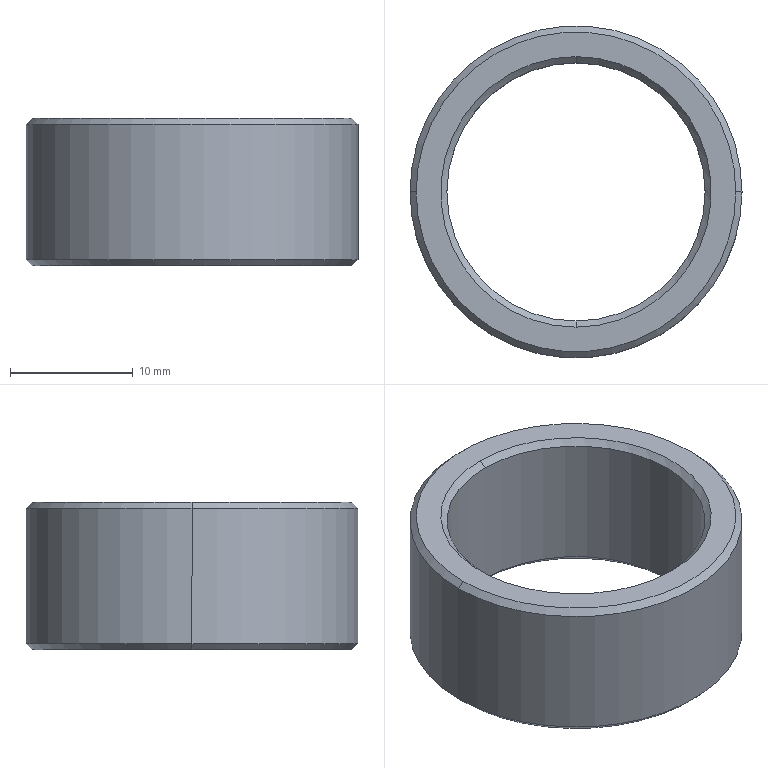Part | STEP file | 1 solid | 14 faces | box 27 x 27 x 12 mm | volume 2677 mm3 | cone 8 | cylinder 4 | plane 2 | commonest cylinder face diameters 21 x2 27 x2
STEP:
#1=CARTESIAN_POINT('',(0.,0.,0.));
#2=DIRECTION('',(0.,0.,1.));
#3=DIRECTION('',(1.,0.,0.));
#4=AXIS2_PLACEMENT_3D('',#1,#2,#3);
#5=CARTESIAN_POINT('',(0.,10.5,0.5));
#6=VERTEX_POINT('',#5);
#7=CARTESIAN_POINT('',(10.5,0.,0.5));
#8=VERTEX_POINT('',#7);
#9=CARTESIAN_POINT('',(0.,0.,0.5));
#10=DIRECTION('',(0.,0.,-1.));
#11=DIRECTION('',(-1.,0.,0.));
#12=AXIS2_PLACEMENT_3D('',#9,#10,#11);
#13=CIRCLE('',#12,10.5);
#14=CARTESIAN_POINT('',(0.,0.,12.));
#15=DIRECTION('',(0.,0.,-1.));
#16=DIRECTION('',(-1.,0.,0.));
#17=AXIS2_PLACEMENT_3D('',#14,#15,#16);
#18=CYLINDRICAL_SURFACE('',#17,10.5);
#19=CARTESIAN_POINT('',(0.,11.5));
#20=DIRECTION('',(1.,0.));
#21=VECTOR('',#20,1.);
#22=LINE('',#19,#21);
#23=(GEOMETRIC_REPRESENTATION_CONTEXT(2)PARAMETRIC_REPRESENTATION_CONTEXT()REPRESENTATION_CONTEXT('',''));
#24=DEFINITIONAL_REPRESENTATION('',(#22),#23);
#25=PCURVE('',#18,#24);
#26=CARTESIAN_POINT('',(0.,0.,0.));
#27=DIRECTION('',(0.,0.,-1.));
#28=DIRECTION('',(0.,1.,0.));
#29=AXIS2_PLACEMENT_3D('',#26,#27,#28);
#30=CONICAL_SURFACE('',#29,11.,0.7854);
#31=CARTESIAN_POINT('',(-1.571,-0.5));
#32=DIRECTION('',(1.,0.));
#33=VECTOR('',#32,1.);
#34=LINE('',#31,#33);
#35=(GEOMETRIC_REPRESENTATION_CONTEXT(2)PARAMETRIC_REPRESENTATION_CONTEXT()REPRESENTATION_CONTEXT('',''));
#36=DEFINITIONAL_REPRESENTATION('',(#34),#35);
#37=PCURVE('',#30,#36);
#38=SURFACE_CURVE('',#13,(#25,#37),.PCURVE_S1.);
#39=EDGE_CURVE('',#6,#8,#38,.T.);
#40=ORIENTED_EDGE('',*,*,#39,.F.);
#41=CARTESIAN_POINT('',(-10.5,0.,0.5));
#42=VERTEX_POINT('',#41);
#43=CARTESIAN_POINT('',(0.,0.,0.5));
#44=DIRECTION('',(0.,0.,-1.));
#45=DIRECTION('',(-1.,0.,0.));
#46=AXIS2_PLACEMENT_3D('',#43,#44,#45);
#47=CIRCLE('',#46,10.5);
#48=CARTESIAN_POINT('',(0.,11.5));
#49=DIRECTION('',(1.,0.));
#50=VECTOR('',#49,1.);
#51=LINE('',#48,#50);
#52=(GEOMETRIC_REPRESENTATION_CONTEXT(2)PARAMETRIC_REPRESENTATION_CONTEXT()REPRESENTATION_CONTEXT('',''));
#53=DEFINITIONAL_REPRESENTATION('',(#51),#52);
#54=PCURVE('',#18,#53);
#55=CARTESIAN_POINT('',(0.,0.,0.));
#56=DIRECTION('',(0.,0.,-1.));
#57=DIRECTION('',(0.,1.,0.));
#58=AXIS2_PLACEMENT_3D('',#55,#56,#57);
#59=CONICAL_SURFACE('',#58,11.,0.7854);
#60=CARTESIAN_POINT('',(4.712,-0.5));
#61=DIRECTION('',(1.,0.));
#62=VECTOR('',#61,1.);
#63=LINE('',#60,#62);
#64=(GEOMETRIC_REPRESENTATION_CONTEXT(2)PARAMETRIC_REPRESENTATION_CONTEXT()REPRESENTATION_CONTEXT('',''));
#65=DEFINITIONAL_REPRESENTATION('',(#63),#64);
#66=PCURVE('',#59,#65);
#67=SURFACE_CURVE('',#47,(#54,#66),.PCURVE_S1.);
#68=EDGE_CURVE('',#42,#6,#67,.T.);
#69=ORIENTED_EDGE('',*,*,#68,.F.);
#70=CARTESIAN_POINT('',(-10.5,0.,11.5));
#71=VERTEX_POINT('',#70);
#72=CARTESIAN_POINT('',(-10.5,0.,12.));
#73=DIRECTION('',(0.,0.,-1.));
#74=VECTOR('',#73,1.);
#75=LINE('',#72,#74);
#76=CARTESIAN_POINT('',(0.,0.));
#77=DIRECTION('',(0.,1.));
#78=VECTOR('',#77,1.);
#79=LINE('',#76,#78);
#80=(GEOMETRIC_REPRESENTATION_CONTEXT(2)PARAMETRIC_REPRESENTATION_CONTEXT()REPRESENTATION_CONTEXT('',''));
#81=DEFINITIONAL_REPRESENTATION('',(#79),#80);
#82=PCURVE('',#18,#81);
#83=CARTESIAN_POINT('',(0.,0.,12.));
#84=DIRECTION('',(0.,0.,-1.));
#85=DIRECTION('',(-1.,0.,0.));
#86=AXIS2_PLACEMENT_3D('',#83,#84,#85);
#87=CYLINDRICAL_SURFACE('',#86,10.5);
#88=CARTESIAN_POINT('',(6.283,0.));
#89=DIRECTION('',(0.,1.));
#90=VECTOR('',#89,1.);
#91=LINE('',#88,#90);
#92=(GEOMETRIC_REPRESENTATION_CONTEXT(2)PARAMETRIC_REPRESENTATION_CONTEXT()REPRESENTATION_CONTEXT('',''));
#93=DEFINITIONAL_REPRESENTATION('',(#91),#92);
#94=PCURVE('',#87,#93);
#95=SURFACE_CURVE('',#75,(#82,#94),.PCURVE_S1.);
#96=EDGE_CURVE('',#71,#42,#95,.T.);
#97=ORIENTED_EDGE('',*,*,#96,.F.);
#98=CARTESIAN_POINT('',(0.,10.5,11.5));
#99=VERTEX_POINT('',#98);
#100=CARTESIAN_POINT('',(0.,0.,11.5));
#101=DIRECTION('',(0.,0.,1.));
#102=DIRECTION('',(1.,0.,0.));
#103=AXIS2_PLACEMENT_3D('',#100,#101,#102);
#104=CIRCLE('',#103,10.5);
#105=CARTESIAN_POINT('',(3.142,0.5));
#106=DIRECTION('',(-1.,0.));
#107=VECTOR('',#106,1.);
#108=LINE('',#105,#107);
#109=(GEOMETRIC_REPRESENTATION_CONTEXT(2)PARAMETRIC_REPRESENTATION_CONTEXT()REPRESENTATION_CONTEXT('',''));
#110=DEFINITIONAL_REPRESENTATION('',(#108),#109);
#111=PCURVE('',#18,#110);
#112=CARTESIAN_POINT('',(0.,0.,12.));
#113=DIRECTION('',(0.,0.,1.));
#114=DIRECTION('',(0.,-1.,0.));
#115=AXIS2_PLACEMENT_3D('',#112,#113,#114);
#116=CONICAL_SURFACE('',#115,11.,0.7854);
#117=CARTESIAN_POINT('',(1.571,-0.5));
#118=DIRECTION('',(1.,0.));
#119=VECTOR('',#118,1.);
#120=LINE('',#117,#119);
#121=(GEOMETRIC_REPRESENTATION_CONTEXT(2)PARAMETRIC_REPRESENTATION_CONTEXT()REPRESENTATION_CONTEXT('',''));
#122=DEFINITIONAL_REPRESENTATION('',(#120),#121);
#123=PCURVE('',#116,#122);
#124=SURFACE_CURVE('',#104,(#111,#123),.PCURVE_S1.);
#125=EDGE_CURVE('',#99,#71,#124,.T.);
#126=ORIENTED_EDGE('',*,*,#125,.F.);
#127=CARTESIAN_POINT('',(10.5,0.,11.5));
#128=VERTEX_POINT('',#127);
#129=CARTESIAN_POINT('',(0.,0.,11.5));
#130=DIRECTION('',(0.,0.,1.));
#131=DIRECTION('',(1.,0.,0.));
#132=AXIS2_PLACEMENT_3D('',#129,#130,#131);
#133=CIRCLE('',#132,10.5);
#134=CARTESIAN_POINT('',(3.142,0.5));
#135=DIRECTION('',(-1.,0.));
#136=VECTOR('',#135,1.);
#137=LINE('',#134,#136);
#138=(GEOMETRIC_REPRESENTATION_CONTEXT(2)PARAMETRIC_REPRESENTATION_CONTEXT()REPRESENTATION_CONTEXT('',''));
#139=DEFINITIONAL_REPRESENTATION('',(#137),#138);
#140=PCURVE('',#18,#139);
#141=CARTESIAN_POINT('',(0.,0.,12.));
#142=DIRECTION('',(0.,0.,1.));
#143=DIRECTION('',(0.,-1.,0.));
#144=AXIS2_PLACEMENT_3D('',#141,#142,#143);
#145=CONICAL_SURFACE('',#144,11.,0.7854);
#146=CARTESIAN_POINT('',(1.571,-0.5));
#147=DIRECTION('',(1.,0.));
#148=VECTOR('',#147,1.);
#149=LINE('',#146,#148);
#150=(GEOMETRIC_REPRESENTATION_CONTEXT(2)PARAMETRIC_REPRESENTATION_CONTEXT()REPRESENTATION_CONTEXT('',''));
#151=DEFINITIONAL_REPRESENTATION('',(#149),#150);
#152=PCURVE('',#145,#151);
#153=SURFACE_CURVE('',#133,(#140,#152),.PCURVE_S1.);
#154=EDGE_CURVE('',#128,#99,#153,.T.);
#155=ORIENTED_EDGE('',*,*,#154,.F.);
#156=CARTESIAN_POINT('',(10.5,0.,12.));
#157=DIRECTION('',(0.,0.,-1.));
#158=VECTOR('',#157,1.);
#159=LINE('',#156,#158);
#160=CARTESIAN_POINT('',(3.142,0.));
#161=DIRECTION('',(0.,1.));
#162=VECTOR('',#161,1.);
#163=LINE('',#160,#162);
#164=(GEOMETRIC_REPRESENTATION_CONTEXT(2)PARAMETRIC_REPRESENTATION_CONTEXT()REPRESENTATION_CONTEXT('',''));
#165=DEFINITIONAL_REPRESENTATION('',(#163),#164);
#166=PCURVE('',#18,#165);
#167=CARTESIAN_POINT('',(3.142,0.));
#168=DIRECTION('',(0.,1.));
#169=VECTOR('',#168,1.);
#170=LINE('',#167,#169);
#171=(GEOMETRIC_REPRESENTATION_CONTEXT(2)PARAMETRIC_REPRESENTATION_CONTEXT()REPRESENTATION_CONTEXT('',''));
#172=DEFINITIONAL_REPRESENTATION('',(#170),#171);
#173=PCURVE('',#87,#172);
#174=SURFACE_CURVE('',#159,(#166,#173),.PCURVE_S1.);
#175=EDGE_CURVE('',#128,#8,#174,.T.);
#176=ORIENTED_EDGE('',*,*,#175,.T.);
#177=EDGE_LOOP('',(#40,#69,#97,#126,#155,#176));
#178=FACE_BOUND('',#177,.F.);
#179=ADVANCED_FACE('',(#178),#18,.F.);
#180=CARTESIAN_POINT('',(0.,11.,12.));
#181=VERTEX_POINT('',#180);
#182=CARTESIAN_POINT('',(0.,-11.,12.));
#183=VERTEX_POINT('',#182);
#184=CARTESIAN_POINT('',(0.,0.,12.));
#185=DIRECTION('',(0.,0.,-1.));
#186=DIRECTION('',(0.,-1.,0.));
#187=AXIS2_PLACEMENT_3D('',#184,#185,#186);
#188=CIRCLE('',#187,11.);
#189=CARTESIAN_POINT('',(6.283,0.));
#190=DIRECTION('',(-1.,0.));
#191=VECTOR('',#190,1.);
#192=LINE('',#189,#191);
#193=(GEOMETRIC_REPRESENTATION_CONTEXT(2)PARAMETRIC_REPRESENTATION_CONTEXT()REPRESENTATION_CONTEXT('',''));
#194=DEFINITIONAL_REPRESENTATION('',(#192),#193);
#195=PCURVE('',#145,#194);
#196=CARTESIAN_POINT('',(0.,0.,12.));
#197=DIRECTION('',(0.,0.,1.));
#198=DIRECTION('',(1.,0.,0.));
#199=AXIS2_PLACEMENT_3D('',#196,#197,#198);
#200=PLANE('',#199);
#201=CARTESIAN_POINT('',(0.,-11.));
#202=CARTESIAN_POINT('',(-19.053,-11.));
#203=CARTESIAN_POINT('',(-9.526,5.5));
#204=CARTESIAN_POINT('',(0.,22.));
#205=CARTESIAN_POINT('',(9.526,5.5));
#206=CARTESIAN_POINT('',(19.053,-11.));
#207=CARTESIAN_POINT('',(0.,-11.));
#208=(BOUNDED_CURVE()B_SPLINE_CURVE(2,(#201,#202,#203,#204,#205,#206,#207),.UNSPECIFIED.,.T.,.F.)B_SPLINE_CURVE_WITH_KNOTS((1,2,2,2,2,1),(-2.094,0.,2.094,4.189,6.283,8.378),.UNSPECIFIED.)CURVE()GEOMETRIC_REPRESENTATION_ITEM()RATIONAL_B_SPLINE_CURVE((1.,0.5,1.,0.5,1.,0.5,1.))REPRESENTATION_ITEM(''));
#209=(GEOMETRIC_REPRESENTATION_CONTEXT(2)PARAMETRIC_REPRESENTATION_CONTEXT()REPRESENTATION_CONTEXT('',''));
#210=DEFINITIONAL_REPRESENTATION('',(#208),#209);
#211=PCURVE('',#200,#210);
#212=SURFACE_CURVE('',#188,(#195,#211),.PCURVE_S1.);
#213=EDGE_CURVE('',#181,#183,#212,.T.);
#214=ORIENTED_EDGE('',*,*,#213,.T.);
#215=CARTESIAN_POINT('',(0.,-10.5,11.5));
#216=VERTEX_POINT('',#215);
#217=CARTESIAN_POINT('',(0.,-11.,12.));
#218=DIRECTION('',(0.,-0.7071,0.7071));
#219=VECTOR('',#218,1.);
#220=LINE('',#217,#219);
#221=CARTESIAN_POINT('',(0.,0.));
#222=DIRECTION('',(0.,1.));
#223=VECTOR('',#222,1.);
#224=LINE('',#221,#223);
#225=(GEOMETRIC_REPRESENTATION_CONTEXT(2)PARAMETRIC_REPRESENTATION_CONTEXT()REPRESENTATION_CONTEXT('',''));
#226=DEFINITIONAL_REPRESENTATION('',(#224),#225);
#227=PCURVE('',#145,#226);
#228=CARTESIAN_POINT('',(6.283,0.));
#229=DIRECTION('',(0.,1.));
#230=VECTOR('',#229,1.);
#231=LINE('',#228,#230);
#232=(GEOMETRIC_REPRESENTATION_CONTEXT(2)PARAMETRIC_REPRESENTATION_CONTEXT()REPRESENTATION_CONTEXT('',''));
#233=DEFINITIONAL_REPRESENTATION('',(#231),#232);
#234=PCURVE('',#116,#233);
#235=SURFACE_CURVE('',#220,(#227,#234),.PCURVE_S1.);
#236=EDGE_CURVE('',#216,#183,#235,.T.);
#237=ORIENTED_EDGE('',*,*,#236,.F.);
#238=CARTESIAN_POINT('',(0.,0.,11.5));
#239=DIRECTION('',(0.,0.,1.));
#240=DIRECTION('',(1.,0.,0.));
#241=AXIS2_PLACEMENT_3D('',#238,#239,#240);
#242=CIRCLE('',#241,10.5);
#243=CARTESIAN_POINT('',(-4.712,-0.5));
#244=DIRECTION('',(1.,0.));
#245=VECTOR('',#244,1.);
#246=LINE('',#243,#245);
#247=(GEOMETRIC_REPRESENTATION_CONTEXT(2)PARAMETRIC_REPRESENTATION_CONTEXT()REPRESENTATION_CONTEXT('',''));
#248=DEFINITIONAL_REPRESENTATION('',(#246),#247);
#249=PCURVE('',#145,#248);
#250=CARTESIAN_POINT('',(9.425,0.5));
#251=DIRECTION('',(-1.,0.));
#252=VECTOR('',#251,1.);
#253=LINE('',#250,#252);
#254=(GEOMETRIC_REPRESENTATION_CONTEXT(2)PARAMETRIC_REPRESENTATION_CONTEXT()REPRESENTATION_CONTEXT('',''));
#255=DEFINITIONAL_REPRESENTATION('',(#253),#254);
#256=PCURVE('',#87,#255);
#257=SURFACE_CURVE('',#242,(#249,#256),.PCURVE_S1.);
#258=EDGE_CURVE('',#216,#128,#257,.T.);
#259=ORIENTED_EDGE('',*,*,#258,.T.);
#260=ORIENTED_EDGE('',*,*,#154,.T.);
#261=CARTESIAN_POINT('',(0.,11.,12.));
#262=DIRECTION('',(0.,0.7071,0.7071));
#263=VECTOR('',#262,1.);
#264=LINE('',#261,#263);
#265=CARTESIAN_POINT('',(3.142,0.));
#266=DIRECTION('',(0.,1.));
#267=VECTOR('',#266,1.);
#268=LINE('',#265,#267);
#269=(GEOMETRIC_REPRESENTATION_CONTEXT(2)PARAMETRIC_REPRESENTATION_CONTEXT()REPRESENTATION_CONTEXT('',''));
#270=DEFINITIONAL_REPRESENTATION('',(#268),#269);
#271=PCURVE('',#145,#270);
#272=CARTESIAN_POINT('',(3.142,0.));
#273=DIRECTION('',(0.,1.));
#274=VECTOR('',#273,1.);
#275=LINE('',#272,#274);
#276=(GEOMETRIC_REPRESENTATION_CONTEXT(2)PARAMETRIC_REPRESENTATION_CONTEXT()REPRESENTATION_CONTEXT('',''));
#277=DEFINITIONAL_REPRESENTATION('',(#275),#276);
#278=PCURVE('',#116,#277);
#279=SURFACE_CURVE('',#264,(#271,#278),.PCURVE_S1.);
#280=EDGE_CURVE('',#99,#181,#279,.T.);
#281=ORIENTED_EDGE('',*,*,#280,.T.);
#282=EDGE_LOOP('',(#214,#237,#259,#260,#281));
#283=FACE_BOUND('',#282,.F.);
#284=ADVANCED_FACE('',(#283),#145,.F.);
#285=CARTESIAN_POINT('',(0.,11.,0.));
#286=VERTEX_POINT('',#285);
#287=CARTESIAN_POINT('',(0.,-11.,0.));
#288=VERTEX_POINT('',#287);
#289=CARTESIAN_POINT('',(0.,0.,0.));
#290=DIRECTION('',(0.,0.,-1.));
#291=DIRECTION('',(0.,1.,0.));
#292=AXIS2_PLACEMENT_3D('',#289,#290,#291);
#293=CIRCLE('',#292,11.);
#294=CARTESIAN_POINT('',(0.,0.));
#295=DIRECTION('',(1.,0.));
#296=VECTOR('',#295,1.);
#297=LINE('',#294,#296);
#298=(GEOMETRIC_REPRESENTATION_CONTEXT(2)PARAMETRIC_REPRESENTATION_CONTEXT()REPRESENTATION_CONTEXT('',''));
#299=DEFINITIONAL_REPRESENTATION('',(#297),#298);
#300=PCURVE('',#30,#299);
#301=CARTESIAN_POINT('',(0.,0.,0.));
#302=DIRECTION('',(0.,0.,1.));
#303=DIRECTION('',(1.,0.,0.));
#304=AXIS2_PLACEMENT_3D('',#301,#302,#303);
#305=PLANE('',#304);
#306=CARTESIAN_POINT('',(0.,11.));
#307=CARTESIAN_POINT('',(19.053,11.));
#308=CARTESIAN_POINT('',(9.526,-5.5));
#309=CARTESIAN_POINT('',(0.,-22.));
#310=CARTESIAN_POINT('',(-9.526,-5.5));
#311=CARTESIAN_POINT('',(-19.053,11.));
#312=CARTESIAN_POINT('',(0.,11.));
#313=(BOUNDED_CURVE()B_SPLINE_CURVE(2,(#306,#307,#308,#309,#310,#311,#312),.UNSPECIFIED.,.T.,.F.)B_SPLINE_CURVE_WITH_KNOTS((1,2,2,2,2,1),(-2.094,0.,2.094,4.189,6.283,8.378),.UNSPECIFIED.)CURVE()GEOMETRIC_REPRESENTATION_ITEM()RATIONAL_B_SPLINE_CURVE((1.,0.5,1.,0.5,1.,0.5,1.))REPRESENTATION_ITEM(''));
#314=(GEOMETRIC_REPRESENTATION_CONTEXT(2)PARAMETRIC_REPRESENTATION_CONTEXT()REPRESENTATION_CONTEXT('',''));
#315=DEFINITIONAL_REPRESENTATION('',(#313),#314);
#316=PCURVE('',#305,#315);
#317=SURFACE_CURVE('',#293,(#300,#316),.PCURVE_S1.);
#318=EDGE_CURVE('',#286,#288,#317,.T.);
#319=ORIENTED_EDGE('',*,*,#318,.F.);
#320=CARTESIAN_POINT('',(0.,11.,0.));
#321=DIRECTION('',(0.,0.7071,-0.7071));
#322=VECTOR('',#321,1.);
#323=LINE('',#320,#322);
#324=CARTESIAN_POINT('',(0.,0.));
#325=DIRECTION('',(0.,1.));
#326=VECTOR('',#325,1.);
#327=LINE('',#324,#326);
#328=(GEOMETRIC_REPRESENTATION_CONTEXT(2)PARAMETRIC_REPRESENTATION_CONTEXT()REPRESENTATION_CONTEXT('',''));
#329=DEFINITIONAL_REPRESENTATION('',(#327),#328);
#330=PCURVE('',#30,#329);
#331=CARTESIAN_POINT('',(6.283,0.));
#332=DIRECTION('',(0.,1.));
#333=VECTOR('',#332,1.);
#334=LINE('',#331,#333);
#335=(GEOMETRIC_REPRESENTATION_CONTEXT(2)PARAMETRIC_REPRESENTATION_CONTEXT()REPRESENTATION_CONTEXT('',''));
#336=DEFINITIONAL_REPRESENTATION('',(#334),#335);
#337=PCURVE('',#59,#336);
#338=SURFACE_CURVE('',#323,(#330,#337),.PCURVE_S1.);
#339=EDGE_CURVE('',#6,#286,#338,.T.);
#340=ORIENTED_EDGE('',*,*,#339,.F.);
#341=ORIENTED_EDGE('',*,*,#39,.T.);
#342=CARTESIAN_POINT('',(0.,-10.5,0.5));
#343=VERTEX_POINT('',#342);
#344=CARTESIAN_POINT('',(0.,0.,0.5));
#345=DIRECTION('',(0.,0.,-1.));
#346=DIRECTION('',(-1.,0.,0.));
#347=AXIS2_PLACEMENT_3D('',#344,#345,#346);
#348=CIRCLE('',#347,10.5);
#349=CARTESIAN_POINT('',(-1.571,-0.5));
#350=DIRECTION('',(1.,0.));
#351=VECTOR('',#350,1.);
#352=LINE('',#349,#351);
#353=(GEOMETRIC_REPRESENTATION_CONTEXT(2)PARAMETRIC_REPRESENTATION_CONTEXT()REPRESENTATION_CONTEXT('',''));
#354=DEFINITIONAL_REPRESENTATION('',(#352),#353);
#355=PCURVE('',#30,#354);
#356=CARTESIAN_POINT('',(0.,11.5));
#357=DIRECTION('',(1.,0.));
#358=VECTOR('',#357,1.);
#359=LINE('',#356,#358);
#360=(GEOMETRIC_REPRESENTATION_CONTEXT(2)PARAMETRIC_REPRESENTATION_CONTEXT()REPRESENTATION_CONTEXT('',''));
#361=DEFINITIONAL_REPRESENTATION('',(#359),#360);
#362=PCURVE('',#87,#361);
#363=SURFACE_CURVE('',#348,(#355,#362),.PCURVE_S1.);
#364=EDGE_CURVE('',#8,#343,#363,.T.);
#365=ORIENTED_EDGE('',*,*,#364,.T.);
#366=CARTESIAN_POINT('',(0.,-11.,0.));
#367=DIRECTION('',(0.,-0.7071,-0.7071));
#368=VECTOR('',#367,1.);
#369=LINE('',#366,#368);
#370=CARTESIAN_POINT('',(3.142,0.));
#371=DIRECTION('',(0.,1.));
#372=VECTOR('',#371,1.);
#373=LINE('',#370,#372);
#374=(GEOMETRIC_REPRESENTATION_CONTEXT(2)PARAMETRIC_REPRESENTATION_CONTEXT()REPRESENTATION_CONTEXT('',''));
#375=DEFINITIONAL_REPRESENTATION('',(#373),#374);
#376=PCURVE('',#30,#375);
#377=CARTESIAN_POINT('',(3.142,0.));
#378=DIRECTION('',(0.,1.));
#379=VECTOR('',#378,1.);
#380=LINE('',#377,#379);
#381=(GEOMETRIC_REPRESENTATION_CONTEXT(2)PARAMETRIC_REPRESENTATION_CONTEXT()REPRESENTATION_CONTEXT('',''));
#382=DEFINITIONAL_REPRESENTATION('',(#380),#381);
#383=PCURVE('',#59,#382);
#384=SURFACE_CURVE('',#369,(#376,#383),.PCURVE_S1.);
#385=EDGE_CURVE('',#343,#288,#384,.T.);
#386=ORIENTED_EDGE('',*,*,#385,.T.);
#387=EDGE_LOOP('',(#319,#340,#341,#365,#386));
#388=FACE_BOUND('',#387,.F.);
#389=ADVANCED_FACE('',(#388),#30,.F.);
#390=CARTESIAN_POINT('',(0.,0.,12.));
#391=DIRECTION('',(0.,0.,-1.));
#392=DIRECTION('',(0.,-1.,0.));
#393=AXIS2_PLACEMENT_3D('',#390,#391,#392);
#394=CIRCLE('',#393,11.);
#395=CARTESIAN_POINT('',(0.,-11.));
#396=CARTESIAN_POINT('',(-19.053,-11.));
#397=CARTESIAN_POINT('',(-9.526,5.5));
#398=CARTESIAN_POINT('',(0.,22.));
#399=CARTESIAN_POINT('',(9.526,5.5));
#400=CARTESIAN_POINT('',(19.053,-11.));
#401=CARTESIAN_POINT('',(0.,-11.));
#402=(BOUNDED_CURVE()B_SPLINE_CURVE(2,(#395,#396,#397,#398,#399,#400,#401),.UNSPECIFIED.,.T.,.F.)B_SPLINE_CURVE_WITH_KNOTS((1,2,2,2,2,1),(-2.094,0.,2.094,4.189,6.283,8.378),.UNSPECIFIED.)CURVE()GEOMETRIC_REPRESENTATION_ITEM()RATIONAL_B_SPLINE_CURVE((1.,0.5,1.,0.5,1.,0.5,1.))REPRESENTATION_ITEM(''));
#403=(GEOMETRIC_REPRESENTATION_CONTEXT(2)PARAMETRIC_REPRESENTATION_CONTEXT()REPRESENTATION_CONTEXT('',''));
#404=DEFINITIONAL_REPRESENTATION('',(#402),#403);
#405=PCURVE('',#200,#404);
#406=CARTESIAN_POINT('',(6.283,0.));
#407=DIRECTION('',(-1.,0.));
#408=VECTOR('',#407,1.);
#409=LINE('',#406,#408);
#410=(GEOMETRIC_REPRESENTATION_CONTEXT(2)PARAMETRIC_REPRESENTATION_CONTEXT()REPRESENTATION_CONTEXT('',''));
#411=DEFINITIONAL_REPRESENTATION('',(#409),#410);
#412=PCURVE('',#116,#411);
#413=SURFACE_CURVE('',#394,(#405,#412),.PCURVE_S1.);
#414=EDGE_CURVE('',#183,#181,#413,.T.);
#415=ORIENTED_EDGE('',*,*,#414,.T.);
#416=ORIENTED_EDGE('',*,*,#213,.T.);
#417=EDGE_LOOP('',(#415,#416));
#418=FACE_BOUND('',#417,.T.);
#419=CARTESIAN_POINT('',(-13.,0.,12.));
#420=VERTEX_POINT('',#419);
#421=CARTESIAN_POINT('',(13.,0.,12.));
#422=VERTEX_POINT('',#421);
#423=CARTESIAN_POINT('',(0.,0.,12.));
#424=DIRECTION('',(0.,0.,-1.));
#425=DIRECTION('',(-1.,0.,0.));
#426=AXIS2_PLACEMENT_3D('',#423,#424,#425);
#427=CIRCLE('',#426,13.);
#428=CARTESIAN_POINT('',(-13.,0.));
#429=CARTESIAN_POINT('',(-13.,22.517));
#430=CARTESIAN_POINT('',(6.5,11.258));
#431=CARTESIAN_POINT('',(26.,0.));
#432=CARTESIAN_POINT('',(6.5,-11.258));
#433=CARTESIAN_POINT('',(-13.,-22.517));
#434=CARTESIAN_POINT('',(-13.,0.));
#435=(BOUNDED_CURVE()B_SPLINE_CURVE(2,(#428,#429,#430,#431,#432,#433,#434),.UNSPECIFIED.,.T.,.F.)B_SPLINE_CURVE_WITH_KNOTS((1,2,2,2,2,1),(-2.094,0.,2.094,4.189,6.283,8.378),.UNSPECIFIED.)CURVE()GEOMETRIC_REPRESENTATION_ITEM()RATIONAL_B_SPLINE_CURVE((1.,0.5,1.,0.5,1.,0.5,1.))REPRESENTATION_ITEM(''));
#436=(GEOMETRIC_REPRESENTATION_CONTEXT(2)PARAMETRIC_REPRESENTATION_CONTEXT()REPRESENTATION_CONTEXT('',''));
#437=DEFINITIONAL_REPRESENTATION('',(#435),#436);
#438=PCURVE('',#200,#437);
#439=CARTESIAN_POINT('',(0.,0.,11.5));
#440=DIRECTION('',(0.,0.,-1.));
#441=DIRECTION('',(-1.,0.,0.));
#442=AXIS2_PLACEMENT_3D('',#439,#440,#441);
#443=CONICAL_SURFACE('',#442,13.5,0.7854);
#444=CARTESIAN_POINT('',(0.,-0.5));
#445=DIRECTION('',(1.,0.));
#446=VECTOR('',#445,1.);
#447=LINE('',#444,#446);
#448=(GEOMETRIC_REPRESENTATION_CONTEXT(2)PARAMETRIC_REPRESENTATION_CONTEXT()REPRESENTATION_CONTEXT('',''));
#449=DEFINITIONAL_REPRESENTATION('',(#447),#448);
#450=PCURVE('',#443,#449);
#451=SURFACE_CURVE('',#427,(#438,#450),.PCURVE_S1.);
#452=EDGE_CURVE('',#420,#422,#451,.T.);
#453=ORIENTED_EDGE('',*,*,#452,.F.);
#454=CARTESIAN_POINT('',(0.,0.,12.));
#455=DIRECTION('',(0.,0.,-1.));
#456=DIRECTION('',(-1.,0.,0.));
#457=AXIS2_PLACEMENT_3D('',#454,#455,#456);
#458=CIRCLE('',#457,13.);
#459=CARTESIAN_POINT('',(-13.,0.));
#460=CARTESIAN_POINT('',(-13.,22.517));
#461=CARTESIAN_POINT('',(6.5,11.258));
#462=CARTESIAN_POINT('',(26.,0.));
#463=CARTESIAN_POINT('',(6.5,-11.258));
#464=CARTESIAN_POINT('',(-13.,-22.517));
#465=CARTESIAN_POINT('',(-13.,0.));
#466=(BOUNDED_CURVE()B_SPLINE_CURVE(2,(#459,#460,#461,#462,#463,#464,#465),.UNSPECIFIED.,.T.,.F.)B_SPLINE_CURVE_WITH_KNOTS((1,2,2,2,2,1),(-2.094,0.,2.094,4.189,6.283,8.378),.UNSPECIFIED.)CURVE()GEOMETRIC_REPRESENTATION_ITEM()RATIONAL_B_SPLINE_CURVE((1.,0.5,1.,0.5,1.,0.5,1.))REPRESENTATION_ITEM(''));
#467=(GEOMETRIC_REPRESENTATION_CONTEXT(2)PARAMETRIC_REPRESENTATION_CONTEXT()REPRESENTATION_CONTEXT('',''));
#468=DEFINITIONAL_REPRESENTATION('',(#466),#467);
#469=PCURVE('',#200,#468);
#470=CARTESIAN_POINT('',(0.,0.,11.5));
#471=DIRECTION('',(0.,0.,-1.));
#472=DIRECTION('',(-1.,0.,0.));
#473=AXIS2_PLACEMENT_3D('',#470,#471,#472);
#474=CONICAL_SURFACE('',#473,13.5,0.7854);
#475=CARTESIAN_POINT('',(0.,-0.5));
#476=DIRECTION('',(1.,0.));
#477=VECTOR('',#476,1.);
#478=LINE('',#475,#477);
#479=(GEOMETRIC_REPRESENTATION_CONTEXT(2)PARAMETRIC_REPRESENTATION_CONTEXT()REPRESENTATION_CONTEXT('',''));
#480=DEFINITIONAL_REPRESENTATION('',(#478),#479);
#481=PCURVE('',#474,#480);
#482=SURFACE_CURVE('',#458,(#469,#481),.PCURVE_S1.);
#483=EDGE_CURVE('',#422,#420,#482,.T.);
#484=ORIENTED_EDGE('',*,*,#483,.F.);
#485=EDGE_LOOP('',(#453,#484));
#486=FACE_BOUND('',#485,.T.);
#487=ADVANCED_FACE('',(#418,#486),#200,.T.);
#488=ORIENTED_EDGE('',*,*,#318,.F.);
#489=CARTESIAN_POINT('',(0.,0.,0.));
#490=DIRECTION('',(0.,0.,-1.));
#491=DIRECTION('',(0.,1.,0.));
#492=AXIS2_PLACEMENT_3D('',#489,#490,#491);
#493=CIRCLE('',#492,11.);
#494=CARTESIAN_POINT('',(0.,11.));
#495=CARTESIAN_POINT('',(19.053,11.));
#496=CARTESIAN_POINT('',(9.526,-5.5));
#497=CARTESIAN_POINT('',(0.,-22.));
#498=CARTESIAN_POINT('',(-9.526,-5.5));
#499=CARTESIAN_POINT('',(-19.053,11.));
#500=CARTESIAN_POINT('',(0.,11.));
#501=(BOUNDED_CURVE()B_SPLINE_CURVE(2,(#494,#495,#496,#497,#498,#499,#500),.UNSPECIFIED.,.T.,.F.)B_SPLINE_CURVE_WITH_KNOTS((1,2,2,2,2,1),(-2.094,0.,2.094,4.189,6.283,8.378),.UNSPECIFIED.)CURVE()GEOMETRIC_REPRESENTATION_ITEM()RATIONAL_B_SPLINE_CURVE((1.,0.5,1.,0.5,1.,0.5,1.))REPRESENTATION_ITEM(''));
#502=(GEOMETRIC_REPRESENTATION_CONTEXT(2)PARAMETRIC_REPRESENTATION_CONTEXT()REPRESENTATION_CONTEXT('',''));
#503=DEFINITIONAL_REPRESENTATION('',(#501),#502);
#504=PCURVE('',#305,#503);
#505=CARTESIAN_POINT('',(0.,0.));
#506=DIRECTION('',(1.,0.));
#507=VECTOR('',#506,1.);
#508=LINE('',#505,#507);
#509=(GEOMETRIC_REPRESENTATION_CONTEXT(2)PARAMETRIC_REPRESENTATION_CONTEXT()REPRESENTATION_CONTEXT('',''));
#510=DEFINITIONAL_REPRESENTATION('',(#508),#509);
#511=PCURVE('',#59,#510);
#512=SURFACE_CURVE('',#493,(#504,#511),.PCURVE_S1.);
#513=EDGE_CURVE('',#288,#286,#512,.T.);
#514=ORIENTED_EDGE('',*,*,#513,.F.);
#515=EDGE_LOOP('',(#488,#514));
#516=FACE_BOUND('',#515,.T.);
#517=CARTESIAN_POINT('',(13.,0.,0.));
#518=VERTEX_POINT('',#517);
#519=CARTESIAN_POINT('',(-13.,0.,0.));
#520=VERTEX_POINT('',#519);
#521=CARTESIAN_POINT('',(0.,0.,0.));
#522=DIRECTION('',(0.,0.,1.));
#523=DIRECTION('',(1.,0.,0.));
#524=AXIS2_PLACEMENT_3D('',#521,#522,#523);
#525=CIRCLE('',#524,13.);
#526=CARTESIAN_POINT('',(0.,0.));
#527=DIRECTION('',(1.,0.));
#528=AXIS2_PLACEMENT_2D('',#526,#527);
#529=CIRCLE('',#528,13.);
#530=(GEOMETRIC_REPRESENTATION_CONTEXT(2)PARAMETRIC_REPRESENTATION_CONTEXT()REPRESENTATION_CONTEXT('',''));
#531=DEFINITIONAL_REPRESENTATION('',(#529),#530);
#532=PCURVE('',#305,#531);
#533=CARTESIAN_POINT('',(0.,0.,0.5));
#534=DIRECTION('',(0.,0.,1.));
#535=DIRECTION('',(1.,0.,0.));
#536=AXIS2_PLACEMENT_3D('',#533,#534,#535);
#537=CONICAL_SURFACE('',#536,13.5,0.7854);
#538=CARTESIAN_POINT('',(0.,-0.5));
#539=DIRECTION('',(1.,0.));
#540=VECTOR('',#539,1.);
#541=LINE('',#538,#540);
#542=(GEOMETRIC_REPRESENTATION_CONTEXT(2)PARAMETRIC_REPRESENTATION_CONTEXT()REPRESENTATION_CONTEXT('',''));
#543=DEFINITIONAL_REPRESENTATION('',(#541),#542);
#544=PCURVE('',#537,#543);
#545=SURFACE_CURVE('',#525,(#532,#544),.PCURVE_S1.);
#546=EDGE_CURVE('',#518,#520,#545,.T.);
#547=ORIENTED_EDGE('',*,*,#546,.F.);
#548=CARTESIAN_POINT('',(0.,0.,0.));
#549=DIRECTION('',(0.,0.,1.));
#550=DIRECTION('',(1.,0.,0.));
#551=AXIS2_PLACEMENT_3D('',#548,#549,#550);
#552=CIRCLE('',#551,13.);
#553=CARTESIAN_POINT('',(0.,0.));
#554=DIRECTION('',(1.,0.));
#555=AXIS2_PLACEMENT_2D('',#553,#554);
#556=CIRCLE('',#555,13.);
#557=(GEOMETRIC_REPRESENTATION_CONTEXT(2)PARAMETRIC_REPRESENTATION_CONTEXT()REPRESENTATION_CONTEXT('',''));
#558=DEFINITIONAL_REPRESENTATION('',(#556),#557);
#559=PCURVE('',#305,#558);
#560=CARTESIAN_POINT('',(0.,0.,0.5));
#561=DIRECTION('',(0.,0.,1.));
#562=DIRECTION('',(1.,0.,0.));
#563=AXIS2_PLACEMENT_3D('',#560,#561,#562);
#564=CONICAL_SURFACE('',#563,13.5,0.7854);
#565=CARTESIAN_POINT('',(0.,-0.5));
#566=DIRECTION('',(1.,0.));
#567=VECTOR('',#566,1.);
#568=LINE('',#565,#567);
#569=(GEOMETRIC_REPRESENTATION_CONTEXT(2)PARAMETRIC_REPRESENTATION_CONTEXT()REPRESENTATION_CONTEXT('',''));
#570=DEFINITIONAL_REPRESENTATION('',(#568),#569);
#571=PCURVE('',#564,#570);
#572=SURFACE_CURVE('',#552,(#559,#571),.PCURVE_S1.);
#573=EDGE_CURVE('',#520,#518,#572,.T.);
#574=ORIENTED_EDGE('',*,*,#573,.F.);
#575=EDGE_LOOP('',(#547,#574));
#576=FACE_BOUND('',#575,.T.);
#577=ADVANCED_FACE('',(#516,#576),#305,.F.);
#578=CARTESIAN_POINT('',(13.5,0.,11.5));
#579=VERTEX_POINT('',#578);
#580=CARTESIAN_POINT('',(13.5,0.,11.5));
#581=DIRECTION('',(0.7071,0.,-0.7071));
#582=VECTOR('',#581,1.);
#583=LINE('',#580,#582);
#584=CARTESIAN_POINT('',(3.142,0.));
#585=DIRECTION('',(0.,1.));
#586=VECTOR('',#585,1.);
#587=LINE('',#584,#586);
#588=(GEOMETRIC_REPRESENTATION_CONTEXT(2)PARAMETRIC_REPRESENTATION_CONTEXT()REPRESENTATION_CONTEXT('',''));
#589=DEFINITIONAL_REPRESENTATION('',(#587),#588);
#590=PCURVE('',#474,#589);
#591=CARTESIAN_POINT('',(3.142,0.));
#592=DIRECTION('',(0.,1.));
#593=VECTOR('',#592,1.);
#594=LINE('',#591,#593);
#595=(GEOMETRIC_REPRESENTATION_CONTEXT(2)PARAMETRIC_REPRESENTATION_CONTEXT()REPRESENTATION_CONTEXT('',''));
#596=DEFINITIONAL_REPRESENTATION('',(#594),#595);
#597=PCURVE('',#443,#596);
#598=SURFACE_CURVE('',#583,(#590,#597),.PCURVE_S1.);
#599=EDGE_CURVE('',#422,#579,#598,.T.);
#600=ORIENTED_EDGE('',*,*,#599,.F.);
#601=ORIENTED_EDGE('',*,*,#483,.T.);
#602=CARTESIAN_POINT('',(-13.5,0.,11.5));
#603=VERTEX_POINT('',#602);
#604=CARTESIAN_POINT('',(-13.5,0.,11.5));
#605=DIRECTION('',(-0.7071,0.,-0.7071));
#606=VECTOR('',#605,1.);
#607=LINE('',#604,#606);
#608=CARTESIAN_POINT('',(6.283,0.));
#609=DIRECTION('',(0.,1.));
#610=VECTOR('',#609,1.);
#611=LINE('',#608,#610);
#612=(GEOMETRIC_REPRESENTATION_CONTEXT(2)PARAMETRIC_REPRESENTATION_CONTEXT()REPRESENTATION_CONTEXT('',''));
#613=DEFINITIONAL_REPRESENTATION('',(#611),#612);
#614=PCURVE('',#474,#613);
#615=CARTESIAN_POINT('',(0.,0.));
#616=DIRECTION('',(0.,1.));
#617=VECTOR('',#616,1.);
#618=LINE('',#615,#617);
#619=(GEOMETRIC_REPRESENTATION_CONTEXT(2)PARAMETRIC_REPRESENTATION_CONTEXT()REPRESENTATION_CONTEXT('',''));
#620=DEFINITIONAL_REPRESENTATION('',(#618),#619);
#621=PCURVE('',#443,#620);
#622=SURFACE_CURVE('',#607,(#614,#621),.PCURVE_S1.);
#623=EDGE_CURVE('',#420,#603,#622,.T.);
#624=ORIENTED_EDGE('',*,*,#623,.T.);
#625=CARTESIAN_POINT('',(0.,0.,11.5));
#626=DIRECTION('',(0.,0.,-1.));
#627=DIRECTION('',(-1.,0.,0.));
#628=AXIS2_PLACEMENT_3D('',#625,#626,#627);
#629=CIRCLE('',#628,13.5);
#630=CARTESIAN_POINT('',(0.,0.));
#631=DIRECTION('',(1.,0.));
#632=VECTOR('',#631,1.);
#633=LINE('',#630,#632);
#634=(GEOMETRIC_REPRESENTATION_CONTEXT(2)PARAMETRIC_REPRESENTATION_CONTEXT()REPRESENTATION_CONTEXT('',''));
#635=DEFINITIONAL_REPRESENTATION('',(#633),#634);
#636=PCURVE('',#474,#635);
#637=CARTESIAN_POINT('',(0.,0.,12.));
#638=DIRECTION('',(0.,0.,-1.));
#639=DIRECTION('',(-1.,0.,0.));
#640=AXIS2_PLACEMENT_3D('',#637,#638,#639);
#641=CYLINDRICAL_SURFACE('',#640,13.5);
#642=CARTESIAN_POINT('',(0.,0.5));
#643=DIRECTION('',(1.,0.));
#644=VECTOR('',#643,1.);
#645=LINE('',#642,#644);
#646=(GEOMETRIC_REPRESENTATION_CONTEXT(2)PARAMETRIC_REPRESENTATION_CONTEXT()REPRESENTATION_CONTEXT('',''));
#647=DEFINITIONAL_REPRESENTATION('',(#645),#646);
#648=PCURVE('',#641,#647);
#649=SURFACE_CURVE('',#629,(#636,#648),.PCURVE_S1.);
#650=EDGE_CURVE('',#579,#603,#649,.T.);
#651=ORIENTED_EDGE('',*,*,#650,.F.);
#652=EDGE_LOOP('',(#600,#601,#624,#651));
#653=FACE_BOUND('',#652,.T.);
#654=ADVANCED_FACE('',(#653),#474,.T.);
#655=CARTESIAN_POINT('',(-13.5,0.,0.5));
#656=VERTEX_POINT('',#655);
#657=CARTESIAN_POINT('',(-13.5,0.,0.5));
#658=DIRECTION('',(-0.7071,0.,0.7071));
#659=VECTOR('',#658,1.);
#660=LINE('',#657,#659);
#661=CARTESIAN_POINT('',(3.142,0.));
#662=DIRECTION('',(0.,1.));
#663=VECTOR('',#662,1.);
#664=LINE('',#661,#663);
#665=(GEOMETRIC_REPRESENTATION_CONTEXT(2)PARAMETRIC_REPRESENTATION_CONTEXT()REPRESENTATION_CONTEXT('',''));
#666=DEFINITIONAL_REPRESENTATION('',(#664),#665);
#667=PCURVE('',#564,#666);
#668=CARTESIAN_POINT('',(3.142,0.));
#669=DIRECTION('',(0.,1.));
#670=VECTOR('',#669,1.);
#671=LINE('',#668,#670);
#672=(GEOMETRIC_REPRESENTATION_CONTEXT(2)PARAMETRIC_REPRESENTATION_CONTEXT()REPRESENTATION_CONTEXT('',''));
#673=DEFINITIONAL_REPRESENTATION('',(#671),#672);
#674=PCURVE('',#537,#673);
#675=SURFACE_CURVE('',#660,(#667,#674),.PCURVE_S1.);
#676=EDGE_CURVE('',#520,#656,#675,.T.);
#677=ORIENTED_EDGE('',*,*,#676,.F.);
#678=ORIENTED_EDGE('',*,*,#573,.T.);
#679=CARTESIAN_POINT('',(13.5,0.,0.5));
#680=VERTEX_POINT('',#679);
#681=CARTESIAN_POINT('',(13.5,0.,0.5));
#682=DIRECTION('',(0.7071,0.,0.7071));
#683=VECTOR('',#682,1.);
#684=LINE('',#681,#683);
#685=CARTESIAN_POINT('',(6.283,0.));
#686=DIRECTION('',(0.,1.));
#687=VECTOR('',#686,1.);
#688=LINE('',#685,#687);
#689=(GEOMETRIC_REPRESENTATION_CONTEXT(2)PARAMETRIC_REPRESENTATION_CONTEXT()REPRESENTATION_CONTEXT('',''));
#690=DEFINITIONAL_REPRESENTATION('',(#688),#689);
#691=PCURVE('',#564,#690);
#692=CARTESIAN_POINT('',(0.,0.));
#693=DIRECTION('',(0.,1.));
#694=VECTOR('',#693,1.);
#695=LINE('',#692,#694);
#696=(GEOMETRIC_REPRESENTATION_CONTEXT(2)PARAMETRIC_REPRESENTATION_CONTEXT()REPRESENTATION_CONTEXT('',''));
#697=DEFINITIONAL_REPRESENTATION('',(#695),#696);
#698=PCURVE('',#537,#697);
#699=SURFACE_CURVE('',#684,(#691,#698),.PCURVE_S1.);
#700=EDGE_CURVE('',#518,#680,#699,.T.);
#701=ORIENTED_EDGE('',*,*,#700,.T.);
#702=CARTESIAN_POINT('',(0.,0.,0.5));
#703=DIRECTION('',(0.,0.,1.));
#704=DIRECTION('',(-1.,0.,0.));
#705=AXIS2_PLACEMENT_3D('',#702,#703,#704);
#706=CIRCLE('',#705,13.5);
#707=CARTESIAN_POINT('',(3.142,0.));
#708=DIRECTION('',(1.,0.));
#709=VECTOR('',#708,1.);
#710=LINE('',#707,#709);
#711=(GEOMETRIC_REPRESENTATION_CONTEXT(2)PARAMETRIC_REPRESENTATION_CONTEXT()REPRESENTATION_CONTEXT('',''));
#712=DEFINITIONAL_REPRESENTATION('',(#710),#711);
#713=PCURVE('',#564,#712);
#714=CARTESIAN_POINT('',(6.283,11.5));
#715=DIRECTION('',(-1.,0.));
#716=VECTOR('',#715,1.);
#717=LINE('',#714,#716);
#718=(GEOMETRIC_REPRESENTATION_CONTEXT(2)PARAMETRIC_REPRESENTATION_CONTEXT()REPRESENTATION_CONTEXT('',''));
#719=DEFINITIONAL_REPRESENTATION('',(#717),#718);
#720=PCURVE('',#641,#719);
#721=SURFACE_CURVE('',#706,(#713,#720),.PCURVE_S1.);
#722=EDGE_CURVE('',#656,#680,#721,.T.);
#723=ORIENTED_EDGE('',*,*,#722,.F.);
#724=EDGE_LOOP('',(#677,#678,#701,#723));
#725=FACE_BOUND('',#724,.T.);
#726=ADVANCED_FACE('',(#725),#564,.T.);
#727=CARTESIAN_POINT('',(13.5,0.,12.));
#728=DIRECTION('',(0.,0.,-1.));
#729=VECTOR('',#728,1.);
#730=LINE('',#727,#729);
#731=CARTESIAN_POINT('',(3.142,0.));
#732=DIRECTION('',(0.,1.));
#733=VECTOR('',#732,1.);
#734=LINE('',#731,#733);
#735=(GEOMETRIC_REPRESENTATION_CONTEXT(2)PARAMETRIC_REPRESENTATION_CONTEXT()REPRESENTATION_CONTEXT('',''));
#736=DEFINITIONAL_REPRESENTATION('',(#734),#735);
#737=PCURVE('',#641,#736);
#738=CARTESIAN_POINT('',(0.,0.,12.));
#739=DIRECTION('',(0.,0.,-1.));
#740=DIRECTION('',(-1.,0.,0.));
#741=AXIS2_PLACEMENT_3D('',#738,#739,#740);
#742=CYLINDRICAL_SURFACE('',#741,13.5);
#743=CARTESIAN_POINT('',(3.142,0.));
#744=DIRECTION('',(0.,1.));
#745=VECTOR('',#744,1.);
#746=LINE('',#743,#745);
#747=(GEOMETRIC_REPRESENTATION_CONTEXT(2)PARAMETRIC_REPRESENTATION_CONTEXT()REPRESENTATION_CONTEXT('',''));
#748=DEFINITIONAL_REPRESENTATION('',(#746),#747);
#749=PCURVE('',#742,#748);
#750=SURFACE_CURVE('',#730,(#737,#749),.PCURVE_S1.);
#751=EDGE_CURVE('',#579,#680,#750,.T.);
#752=ORIENTED_EDGE('',*,*,#751,.F.);
#753=ORIENTED_EDGE('',*,*,#650,.T.);
#754=CARTESIAN_POINT('',(-13.5,0.,12.));
#755=DIRECTION('',(0.,0.,-1.));
#756=VECTOR('',#755,1.);
#757=LINE('',#754,#756);
#758=CARTESIAN_POINT('',(6.283,0.));
#759=DIRECTION('',(0.,1.));
#760=VECTOR('',#759,1.);
#761=LINE('',#758,#760);
#762=(GEOMETRIC_REPRESENTATION_CONTEXT(2)PARAMETRIC_REPRESENTATION_CONTEXT()REPRESENTATION_CONTEXT('',''));
#763=DEFINITIONAL_REPRESENTATION('',(#761),#762);
#764=PCURVE('',#641,#763);
#765=CARTESIAN_POINT('',(0.,0.));
#766=DIRECTION('',(0.,1.));
#767=VECTOR('',#766,1.);
#768=LINE('',#765,#767);
#769=(GEOMETRIC_REPRESENTATION_CONTEXT(2)PARAMETRIC_REPRESENTATION_CONTEXT()REPRESENTATION_CONTEXT('',''));
#770=DEFINITIONAL_REPRESENTATION('',(#768),#769);
#771=PCURVE('',#742,#770);
#772=SURFACE_CURVE('',#757,(#764,#771),.PCURVE_S1.);
#773=EDGE_CURVE('',#603,#656,#772,.T.);
#774=ORIENTED_EDGE('',*,*,#773,.T.);
#775=ORIENTED_EDGE('',*,*,#722,.T.);
#776=EDGE_LOOP('',(#752,#753,#774,#775));
#777=FACE_BOUND('',#776,.T.);
#778=ADVANCED_FACE('',(#777),#641,.T.);
#779=ORIENTED_EDGE('',*,*,#96,.T.);
#780=CARTESIAN_POINT('',(0.,0.,0.5));
#781=DIRECTION('',(0.,0.,-1.));
#782=DIRECTION('',(-1.,0.,0.));
#783=AXIS2_PLACEMENT_3D('',#780,#781,#782);
#784=CIRCLE('',#783,10.5);
#785=CARTESIAN_POINT('',(0.,11.5));
#786=DIRECTION('',(1.,0.));
#787=VECTOR('',#786,1.);
#788=LINE('',#785,#787);
#789=(GEOMETRIC_REPRESENTATION_CONTEXT(2)PARAMETRIC_REPRESENTATION_CONTEXT()REPRESENTATION_CONTEXT('',''));
#790=DEFINITIONAL_REPRESENTATION('',(#788),#789);
#791=PCURVE('',#87,#790);
#792=CARTESIAN_POINT('',(-1.571,-0.5));
#793=DIRECTION('',(1.,0.));
#794=VECTOR('',#793,1.);
#795=LINE('',#792,#794);
#796=(GEOMETRIC_REPRESENTATION_CONTEXT(2)PARAMETRIC_REPRESENTATION_CONTEXT()REPRESENTATION_CONTEXT('',''));
#797=DEFINITIONAL_REPRESENTATION('',(#795),#796);
#798=PCURVE('',#59,#797);
#799=SURFACE_CURVE('',#784,(#791,#798),.PCURVE_S1.);
#800=EDGE_CURVE('',#343,#42,#799,.T.);
#801=ORIENTED_EDGE('',*,*,#800,.F.);
#802=ORIENTED_EDGE('',*,*,#364,.F.);
#803=ORIENTED_EDGE('',*,*,#175,.F.);
#804=ORIENTED_EDGE('',*,*,#258,.F.);
#805=CARTESIAN_POINT('',(0.,0.,11.5));
#806=DIRECTION('',(0.,0.,1.));
#807=DIRECTION('',(1.,0.,0.));
#808=AXIS2_PLACEMENT_3D('',#805,#806,#807);
#809=CIRCLE('',#808,10.5);
#810=CARTESIAN_POINT('',(9.425,0.5));
#811=DIRECTION('',(-1.,0.));
#812=VECTOR('',#811,1.);
#813=LINE('',#810,#812);
#814=(GEOMETRIC_REPRESENTATION_CONTEXT(2)PARAMETRIC_REPRESENTATION_CONTEXT()REPRESENTATION_CONTEXT('',''));
#815=DEFINITIONAL_REPRESENTATION('',(#813),#814);
#816=PCURVE('',#87,#815);
#817=CARTESIAN_POINT('',(1.571,-0.5));
#818=DIRECTION('',(1.,0.));
#819=VECTOR('',#818,1.);
#820=LINE('',#817,#819);
#821=(GEOMETRIC_REPRESENTATION_CONTEXT(2)PARAMETRIC_REPRESENTATION_CONTEXT()REPRESENTATION_CONTEXT('',''));
#822=DEFINITIONAL_REPRESENTATION('',(#820),#821);
#823=PCURVE('',#116,#822);
#824=SURFACE_CURVE('',#809,(#816,#823),.PCURVE_S1.);
#825=EDGE_CURVE('',#71,#216,#824,.T.);
#826=ORIENTED_EDGE('',*,*,#825,.F.);
#827=EDGE_LOOP('',(#779,#801,#802,#803,#804,#826));
#828=FACE_BOUND('',#827,.F.);
#829=ADVANCED_FACE('',(#828),#87,.F.);
#830=ORIENTED_EDGE('',*,*,#825,.T.);
#831=ORIENTED_EDGE('',*,*,#236,.T.);
#832=ORIENTED_EDGE('',*,*,#414,.T.);
#833=ORIENTED_EDGE('',*,*,#280,.F.);
#834=ORIENTED_EDGE('',*,*,#125,.T.);
#835=EDGE_LOOP('',(#830,#831,#832,#833,#834));
#836=FACE_BOUND('',#835,.F.);
#837=ADVANCED_FACE('',(#836),#116,.F.);
#838=ORIENTED_EDGE('',*,*,#68,.T.);
#839=ORIENTED_EDGE('',*,*,#339,.T.);
#840=ORIENTED_EDGE('',*,*,#513,.F.);
#841=ORIENTED_EDGE('',*,*,#385,.F.);
#842=ORIENTED_EDGE('',*,*,#800,.T.);
#843=EDGE_LOOP('',(#838,#839,#840,#841,#842));
#844=FACE_BOUND('',#843,.F.);
#845=ADVANCED_FACE('',(#844),#59,.F.);
#846=ORIENTED_EDGE('',*,*,#452,.T.);
#847=ORIENTED_EDGE('',*,*,#599,.T.);
#848=CARTESIAN_POINT('',(0.,0.,11.5));
#849=DIRECTION('',(0.,0.,-1.));
#850=DIRECTION('',(-1.,0.,0.));
#851=AXIS2_PLACEMENT_3D('',#848,#849,#850);
#852=CIRCLE('',#851,13.5);
#853=CARTESIAN_POINT('',(0.,0.));
#854=DIRECTION('',(1.,0.));
#855=VECTOR('',#854,1.);
#856=LINE('',#853,#855);
#857=(GEOMETRIC_REPRESENTATION_CONTEXT(2)PARAMETRIC_REPRESENTATION_CONTEXT()REPRESENTATION_CONTEXT('',''));
#858=DEFINITIONAL_REPRESENTATION('',(#856),#857);
#859=PCURVE('',#443,#858);
#860=CARTESIAN_POINT('',(0.,0.5));
#861=DIRECTION('',(1.,0.));
#862=VECTOR('',#861,1.);
#863=LINE('',#860,#862);
#864=(GEOMETRIC_REPRESENTATION_CONTEXT(2)PARAMETRIC_REPRESENTATION_CONTEXT()REPRESENTATION_CONTEXT('',''));
#865=DEFINITIONAL_REPRESENTATION('',(#863),#864);
#866=PCURVE('',#742,#865);
#867=SURFACE_CURVE('',#852,(#859,#866),.PCURVE_S1.);
#868=EDGE_CURVE('',#603,#579,#867,.T.);
#869=ORIENTED_EDGE('',*,*,#868,.F.);
#870=ORIENTED_EDGE('',*,*,#623,.F.);
#871=EDGE_LOOP('',(#846,#847,#869,#870));
#872=FACE_BOUND('',#871,.T.);
#873=ADVANCED_FACE('',(#872),#443,.T.);
#874=ORIENTED_EDGE('',*,*,#546,.T.);
#875=ORIENTED_EDGE('',*,*,#676,.T.);
#876=CARTESIAN_POINT('',(0.,0.,0.5));
#877=DIRECTION('',(0.,0.,1.));
#878=DIRECTION('',(-1.,0.,0.));
#879=AXIS2_PLACEMENT_3D('',#876,#877,#878);
#880=CIRCLE('',#879,13.5);
#881=CARTESIAN_POINT('',(-3.142,0.));
#882=DIRECTION('',(1.,0.));
#883=VECTOR('',#882,1.);
#884=LINE('',#881,#883);
#885=(GEOMETRIC_REPRESENTATION_CONTEXT(2)PARAMETRIC_REPRESENTATION_CONTEXT()REPRESENTATION_CONTEXT('',''));
#886=DEFINITIONAL_REPRESENTATION('',(#884),#885);
#887=PCURVE('',#537,#886);
#888=CARTESIAN_POINT('',(6.283,11.5));
#889=DIRECTION('',(-1.,0.));
#890=VECTOR('',#889,1.);
#891=LINE('',#888,#890);
#892=(GEOMETRIC_REPRESENTATION_CONTEXT(2)PARAMETRIC_REPRESENTATION_CONTEXT()REPRESENTATION_CONTEXT('',''));
#893=DEFINITIONAL_REPRESENTATION('',(#891),#892);
#894=PCURVE('',#742,#893);
#895=SURFACE_CURVE('',#880,(#887,#894),.PCURVE_S1.);
#896=EDGE_CURVE('',#680,#656,#895,.T.);
#897=ORIENTED_EDGE('',*,*,#896,.F.);
#898=ORIENTED_EDGE('',*,*,#700,.F.);
#899=EDGE_LOOP('',(#874,#875,#897,#898));
#900=FACE_BOUND('',#899,.T.);
#901=ADVANCED_FACE('',(#900),#537,.T.);
#902=ORIENTED_EDGE('',*,*,#868,.T.);
#903=ORIENTED_EDGE('',*,*,#751,.T.);
#904=ORIENTED_EDGE('',*,*,#896,.T.);
#905=ORIENTED_EDGE('',*,*,#773,.F.);
#906=EDGE_LOOP('',(#902,#903,#904,#905));
#907=FACE_BOUND('',#906,.T.);
#908=ADVANCED_FACE('',(#907),#742,.T.);
#909=CLOSED_SHELL('',(#179,#284,#389,#487,#577,#654,#726,#778,#829,#837,#845,#873,#901,#908));
#910=MANIFOLD_SOLID_BREP('',#909);
#911=(LENGTH_UNIT()NAMED_UNIT(*)SI_UNIT(.MILLI.,.METRE.));
#912=UNCERTAINTY_MEASURE_WITH_UNIT(LENGTH_MEASURE(0.0000001),#911,'','');
#913=(NAMED_UNIT(*)PLANE_ANGLE_UNIT()SI_UNIT($,.RADIAN.));
#914=(NAMED_UNIT(*)SI_UNIT($,.STERADIAN.)SOLID_ANGLE_UNIT());
#915=(GEOMETRIC_REPRESENTATION_CONTEXT(3)GLOBAL_UNCERTAINTY_ASSIGNED_CONTEXT((#912))GLOBAL_UNIT_ASSIGNED_CONTEXT((#911,#913,#914))REPRESENTATION_CONTEXT('',''));
#916=ADVANCED_BREP_SHAPE_REPRESENTATION('',(#4,#910),#915);